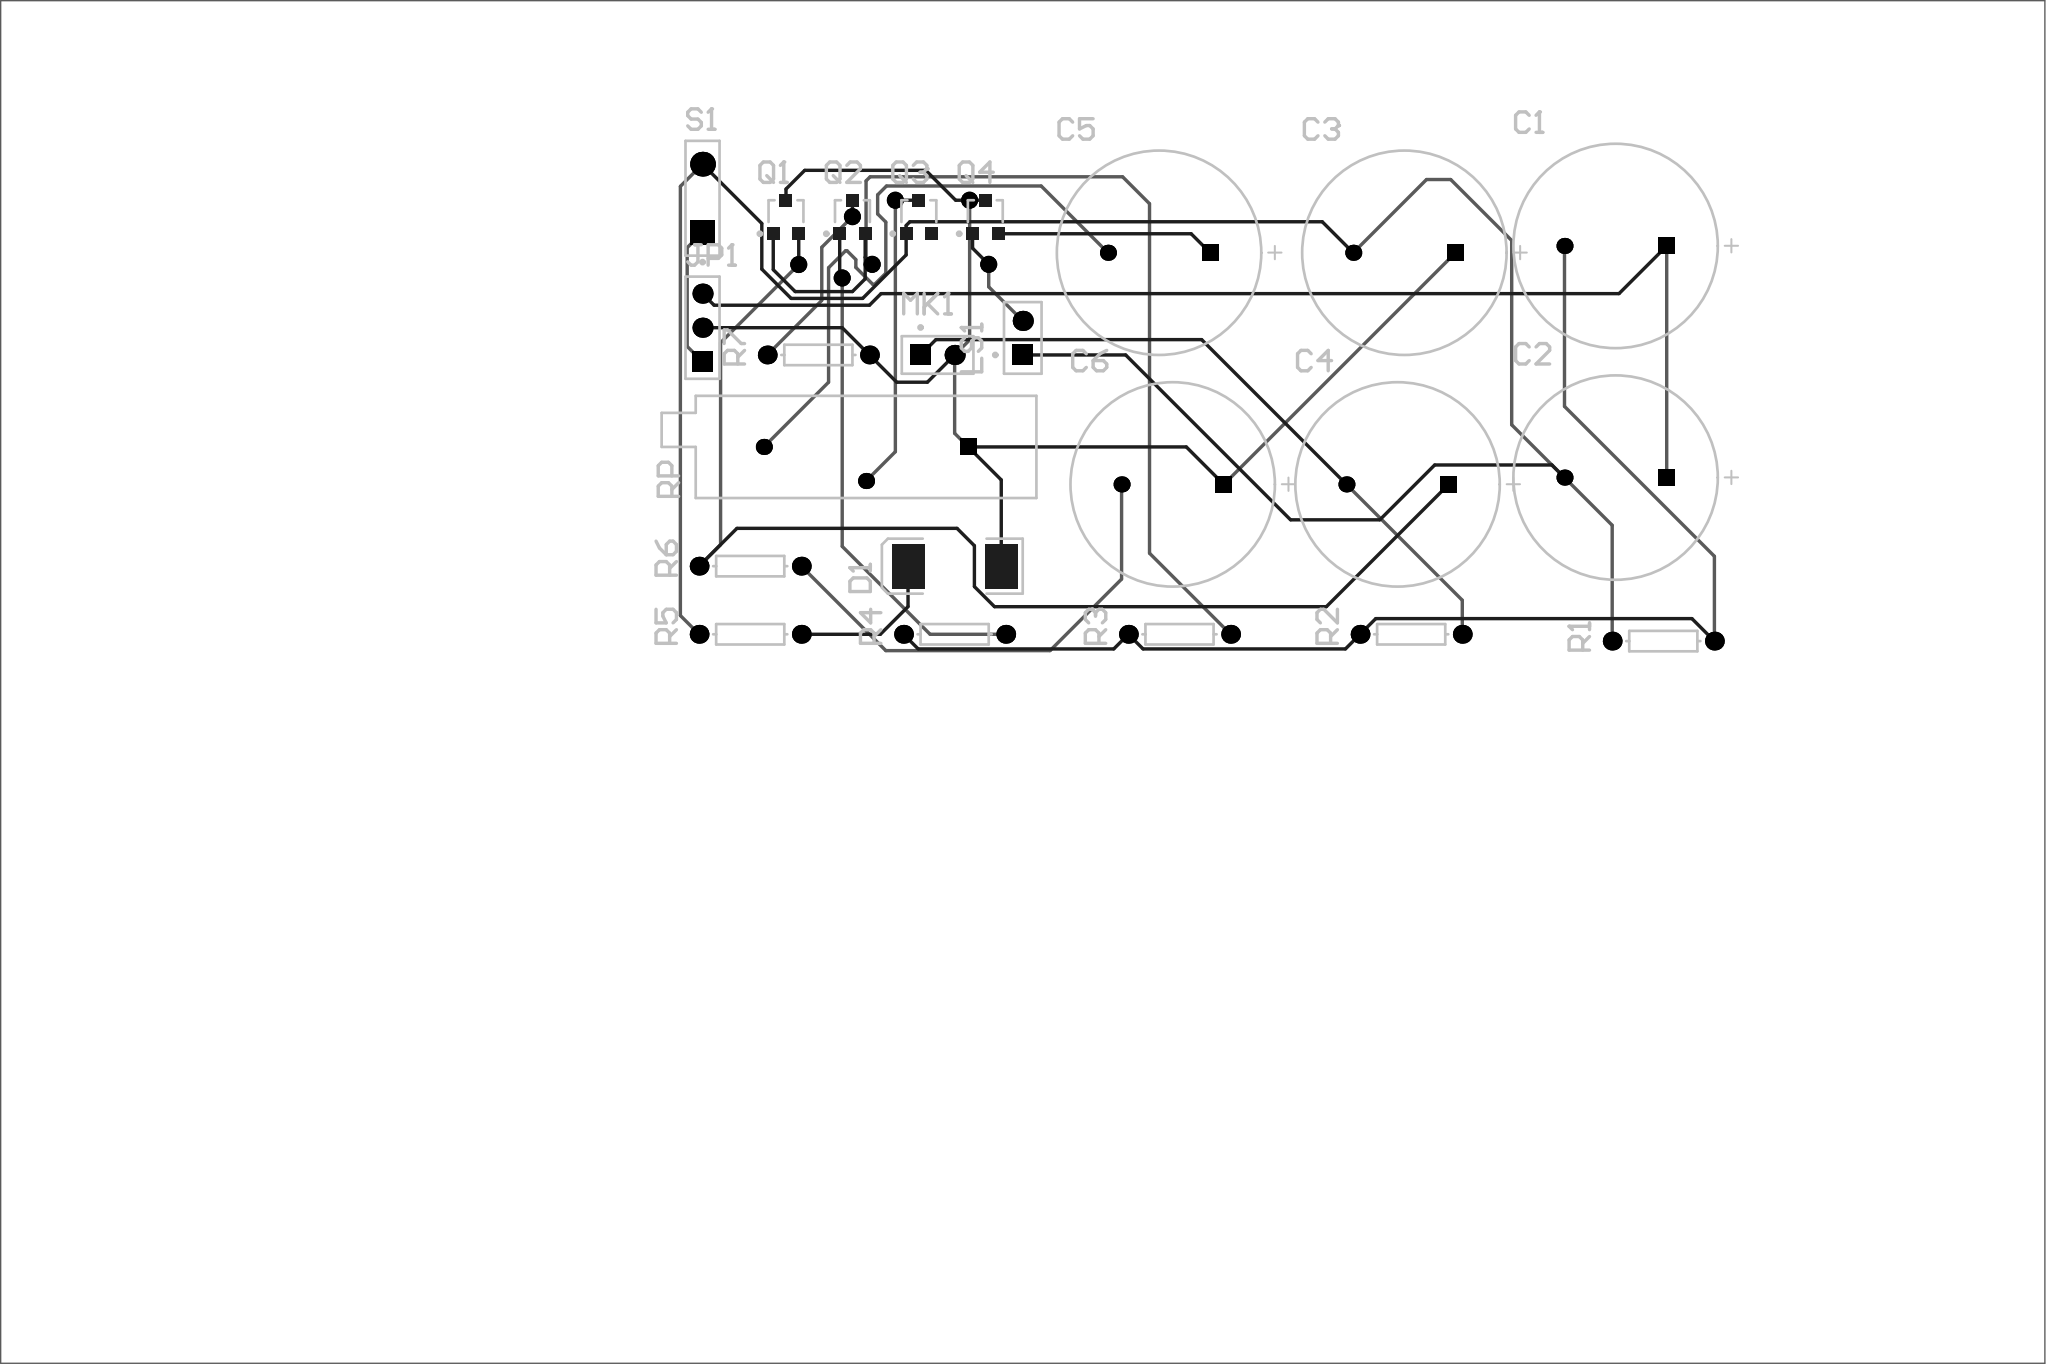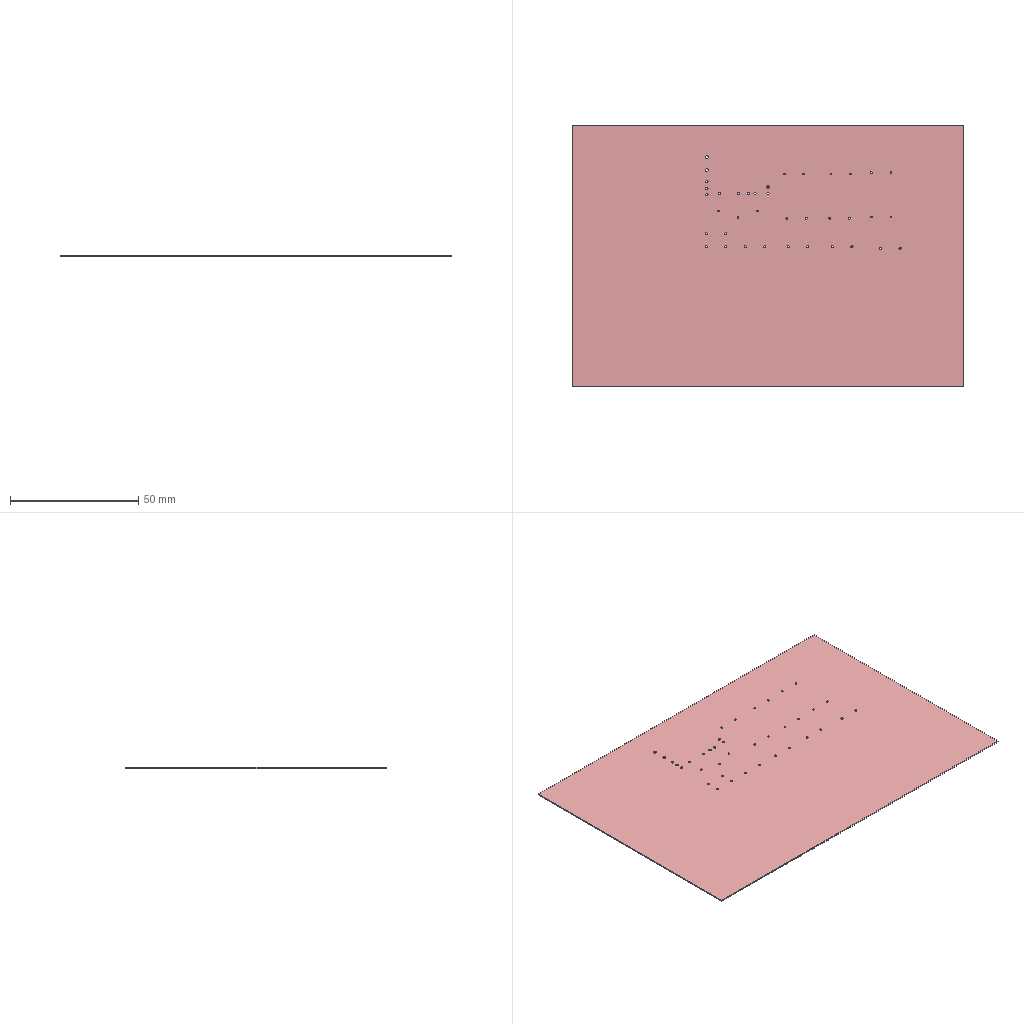Circuit board layout | Altium Designer | box 152.4 x 101.6 x 0.4 mm
Part placement:
Designator,Comment,Layer,Footprint,Center-X(mm),Center-Y(mm),Rotation
C1,Cap Pol1,TopLayer,RB7.6-15,145.796,108.712,0
C2,Cap Pol1,TopLayer,RB7.6-15,145.796,91.44,0
C3,Cap Pol1,TopLayer,RB7.6-15,130.048,108.204,0
C4,Cap Pol1,TopLayer,RB7.6-15,129.54,90.932,0
C5,Cap Pol1,TopLayer,RB7.6-15,111.76,108.204,0
C6,Cap Pol1,TopLayer,RB7.6-15,112.776,90.932,0
D1,Diode,TopLayer,DSO-C2/X3.3,96.52,84.836,180
JP1,Header 3,TopLayer,HDR1X3,77.724,102.616,90
LS1,Speaker,TopLayer,PIN2,101.6,101.854,90
MK1,Mic1,TopLayer,PIN2,95.25,100.584,0
Q1,PNP,TopLayer,SO-G3/C2.5,83.947,110.871,0
Q2,PNP,TopLayer,SO-G3/C2.5,88.9,110.871,0
Q3,PNP,TopLayer,SO-G3/C2.5,93.853,110.871,0
Q4,PNP,TopLayer,SO-G3/C2.5,98.806,110.871,0
R1,Res1,TopLayer,AXIAL-0.3,149.352,79.248,180
R2,Res1,TopLayer,AXIAL-0.3,130.556,79.756,180
R3,Res1,TopLayer,AXIAL-0.3,113.284,79.756,180
R4,Res1,TopLayer,AXIAL-0.3,96.52,79.756,180
R5,Res1,TopLayer,AXIAL-0.3,81.28,79.756,180
R6,Res1,TopLayer,AXIAL-0.3,81.28,84.836,180
R7,Res1,TopLayer,AXIAL-0.3,86.36,100.584,180
RP,RPot,TopLayer,VR2,89.916,92.456,180
S1,SW-SPST,TopLayer,SPST-2,77.724,112.268,90